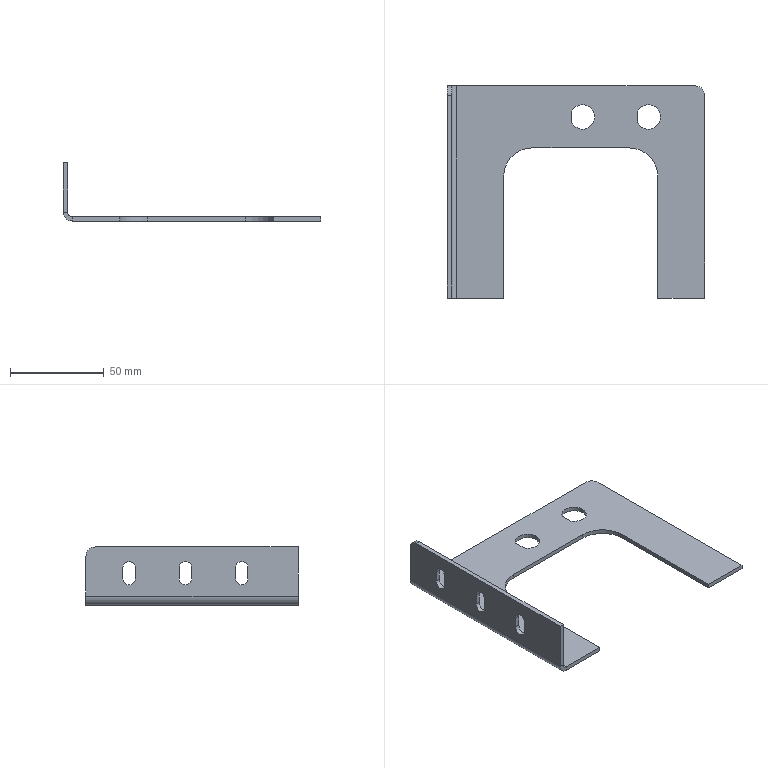Part | SolidWorks | features ICE 2, Fillet 1, FlatPattern 1, SMBaseFlange 1, SheetMetal 1 | 1 solid | 43 faces | box 137 x 113 x 31 mm | volume 26668 mm3 | plane 24 | cylinder 19 | commonest cylinder face diameters 6.6 x9 13 x4 10 x2 30 x2 5 x1 9.6 x1
STEP:
#1=CARTESIAN_POINT('',(2.3,30.,23.25));
#2=VERTEX_POINT('',#1);
#3=CARTESIAN_POINT('',(2.3,33.3,19.95));
#4=VERTEX_POINT('',#3);
#5=CARTESIAN_POINT('',(2.3,30.,19.95));
#6=DIRECTION('',(-1.,0.,0.));
#7=DIRECTION('',(0.,0.,-1.));
#8=AXIS2_PLACEMENT_3D('',#5,#6,#7);
#9=CIRCLE('',#8,3.3);
#10=EDGE_CURVE('',#2,#4,#9,.T.);
#11=ORIENTED_EDGE('',*,*,#10,.F.);
#12=CARTESIAN_POINT('',(0.,30.,23.25));
#13=VERTEX_POINT('',#12);
#14=CARTESIAN_POINT('',(137.001,30.,23.25));
#15=DIRECTION('',(-1.,0.,0.));
#16=VECTOR('',#15,1000.);
#17=LINE('',#14,#16);
#18=EDGE_CURVE('',#2,#13,#17,.T.);
#19=ORIENTED_EDGE('',*,*,#18,.T.);
#20=CARTESIAN_POINT('',(0.,33.3,19.95));
#21=VERTEX_POINT('',#20);
#22=CARTESIAN_POINT('',(0.,30.,19.95));
#23=DIRECTION('',(-1.,0.,0.));
#24=DIRECTION('',(0.,0.,1.));
#25=AXIS2_PLACEMENT_3D('',#22,#23,#24);
#26=CIRCLE('',#25,3.3);
#27=EDGE_CURVE('',#13,#21,#26,.T.);
#28=ORIENTED_EDGE('',*,*,#27,.T.);
#29=CARTESIAN_POINT('',(137.001,33.3,19.95));
#30=DIRECTION('',(-1.,0.,0.));
#31=VECTOR('',#30,1000.);
#32=LINE('',#29,#31);
#33=EDGE_CURVE('',#4,#21,#32,.T.);
#34=ORIENTED_EDGE('',*,*,#33,.F.);
#35=EDGE_LOOP('',(#11,#19,#28,#34));
#36=FACE_OUTER_BOUND('',#35,.T.);
#37=CARTESIAN_POINT('',(137.001,30.,19.95));
#38=DIRECTION('',(-1.,0.,0.));
#39=DIRECTION('',(0.,0.,1.));
#40=AXIS2_PLACEMENT_3D('',#37,#38,#39);
#41=CYLINDRICAL_SURFACE('',#40,3.3);
#42=ADVANCED_FACE('',(#36),#41,.F.);
#43=CARTESIAN_POINT('',(2.3,60.,23.25));
#44=VERTEX_POINT('',#43);
#45=CARTESIAN_POINT('',(2.3,63.3,19.95));
#46=VERTEX_POINT('',#45);
#47=CARTESIAN_POINT('',(2.3,60.,19.95));
#48=DIRECTION('',(-1.,0.,0.));
#49=DIRECTION('',(0.,0.,-1.));
#50=AXIS2_PLACEMENT_3D('',#47,#48,#49);
#51=CIRCLE('',#50,3.3);
#52=EDGE_CURVE('',#44,#46,#51,.T.);
#53=ORIENTED_EDGE('',*,*,#52,.F.);
#54=CARTESIAN_POINT('',(0.,60.,23.25));
#55=VERTEX_POINT('',#54);
#56=CARTESIAN_POINT('',(137.001,60.,23.25));
#57=DIRECTION('',(-1.,0.,0.));
#58=VECTOR('',#57,1000.);
#59=LINE('',#56,#58);
#60=EDGE_CURVE('',#44,#55,#59,.T.);
#61=ORIENTED_EDGE('',*,*,#60,.T.);
#62=CARTESIAN_POINT('',(0.,63.3,19.95));
#63=VERTEX_POINT('',#62);
#64=CARTESIAN_POINT('',(0.,60.,19.95));
#65=DIRECTION('',(-1.,0.,0.));
#66=DIRECTION('',(0.,0.,1.));
#67=AXIS2_PLACEMENT_3D('',#64,#65,#66);
#68=CIRCLE('',#67,3.3);
#69=EDGE_CURVE('',#55,#63,#68,.T.);
#70=ORIENTED_EDGE('',*,*,#69,.T.);
#71=CARTESIAN_POINT('',(137.001,63.3,19.95));
#72=DIRECTION('',(-1.,0.,0.));
#73=VECTOR('',#72,1000.);
#74=LINE('',#71,#73);
#75=EDGE_CURVE('',#46,#63,#74,.T.);
#76=ORIENTED_EDGE('',*,*,#75,.F.);
#77=EDGE_LOOP('',(#53,#61,#70,#76));
#78=FACE_OUTER_BOUND('',#77,.T.);
#79=CARTESIAN_POINT('',(137.001,60.,19.95));
#80=DIRECTION('',(-1.,0.,0.));
#81=DIRECTION('',(0.,0.,1.));
#82=AXIS2_PLACEMENT_3D('',#79,#80,#81);
#83=CYLINDRICAL_SURFACE('',#82,3.3);
#84=ADVANCED_FACE('',(#78),#83,.F.);
#85=CARTESIAN_POINT('',(2.3,90.,23.25));
#86=VERTEX_POINT('',#85);
#87=CARTESIAN_POINT('',(2.3,93.3,19.95));
#88=VERTEX_POINT('',#87);
#89=CARTESIAN_POINT('',(2.3,90.,19.95));
#90=DIRECTION('',(-1.,0.,0.));
#91=DIRECTION('',(0.,0.,-1.));
#92=AXIS2_PLACEMENT_3D('',#89,#90,#91);
#93=CIRCLE('',#92,3.3);
#94=EDGE_CURVE('',#86,#88,#93,.T.);
#95=ORIENTED_EDGE('',*,*,#94,.F.);
#96=CARTESIAN_POINT('',(0.,90.,23.25));
#97=VERTEX_POINT('',#96);
#98=CARTESIAN_POINT('',(137.001,90.,23.25));
#99=DIRECTION('',(-1.,0.,0.));
#100=VECTOR('',#99,1000.);
#101=LINE('',#98,#100);
#102=EDGE_CURVE('',#86,#97,#101,.T.);
#103=ORIENTED_EDGE('',*,*,#102,.T.);
#104=CARTESIAN_POINT('',(0.,93.3,19.95));
#105=VERTEX_POINT('',#104);
#106=CARTESIAN_POINT('',(0.,90.,19.95));
#107=DIRECTION('',(-1.,0.,0.));
#108=DIRECTION('',(0.,0.,1.));
#109=AXIS2_PLACEMENT_3D('',#106,#107,#108);
#110=CIRCLE('',#109,3.3);
#111=EDGE_CURVE('',#97,#105,#110,.T.);
#112=ORIENTED_EDGE('',*,*,#111,.T.);
#113=CARTESIAN_POINT('',(137.001,93.3,19.95));
#114=DIRECTION('',(-1.,0.,0.));
#115=VECTOR('',#114,1000.);
#116=LINE('',#113,#115);
#117=EDGE_CURVE('',#88,#105,#116,.T.);
#118=ORIENTED_EDGE('',*,*,#117,.F.);
#119=EDGE_LOOP('',(#95,#103,#112,#118));
#120=FACE_OUTER_BOUND('',#119,.T.);
#121=CARTESIAN_POINT('',(137.001,90.,19.95));
#122=DIRECTION('',(-1.,0.,0.));
#123=DIRECTION('',(0.,0.,1.));
#124=AXIS2_PLACEMENT_3D('',#121,#122,#123);
#125=CYLINDRICAL_SURFACE('',#124,3.3);
#126=ADVANCED_FACE('',(#120),#125,.F.);
#127=CARTESIAN_POINT('',(101.3,99.624,0.));
#128=VERTEX_POINT('',#127);
#129=CARTESIAN_POINT('',(113.5,96.5,0.));
#130=VERTEX_POINT('',#129);
#131=CARTESIAN_POINT('',(107.,96.5,0.));
#132=DIRECTION('',(0.,0.,-1.));
#133=DIRECTION('',(1.,0.,0.));
#134=AXIS2_PLACEMENT_3D('',#131,#132,#133);
#135=CIRCLE('',#134,6.5);
#136=EDGE_CURVE('',#128,#130,#135,.T.);
#137=ORIENTED_EDGE('',*,*,#136,.T.);
#138=CARTESIAN_POINT('',(113.5,96.5,2.3));
#139=VERTEX_POINT('',#138);
#140=CARTESIAN_POINT('',(113.5,96.5,-0.001));
#141=DIRECTION('',(0.,0.,1.));
#142=VECTOR('',#141,1000.);
#143=LINE('',#140,#142);
#144=EDGE_CURVE('',#130,#139,#143,.T.);
#145=ORIENTED_EDGE('',*,*,#144,.T.);
#146=CARTESIAN_POINT('',(101.3,99.624,2.3));
#147=VERTEX_POINT('',#146);
#148=CARTESIAN_POINT('',(107.,96.5,2.3));
#149=DIRECTION('',(0.,0.,1.));
#150=DIRECTION('',(1.,0.,0.));
#151=AXIS2_PLACEMENT_3D('',#148,#149,#150);
#152=CIRCLE('',#151,6.5);
#153=EDGE_CURVE('',#139,#147,#152,.T.);
#154=ORIENTED_EDGE('',*,*,#153,.T.);
#155=CARTESIAN_POINT('',(101.3,99.624,-0.001));
#156=DIRECTION('',(0.,0.,1.));
#157=VECTOR('',#156,1000.);
#158=LINE('',#155,#157);
#159=EDGE_CURVE('',#128,#147,#158,.T.);
#160=ORIENTED_EDGE('',*,*,#159,.F.);
#161=EDGE_LOOP('',(#137,#145,#154,#160));
#162=FACE_OUTER_BOUND('',#161,.T.);
#163=CARTESIAN_POINT('',(107.,96.5,-0.001));
#164=DIRECTION('',(0.,0.,1.));
#165=DIRECTION('',(1.,0.,0.));
#166=AXIS2_PLACEMENT_3D('',#163,#164,#165);
#167=CYLINDRICAL_SURFACE('',#166,6.5);
#168=ADVANCED_FACE('',(#162),#167,.F.);
#169=CARTESIAN_POINT('',(66.3,99.624,0.));
#170=VERTEX_POINT('',#169);
#171=CARTESIAN_POINT('',(78.5,96.5,0.));
#172=VERTEX_POINT('',#171);
#173=CARTESIAN_POINT('',(72.,96.5,0.));
#174=DIRECTION('',(0.,0.,-1.));
#175=DIRECTION('',(1.,0.,0.));
#176=AXIS2_PLACEMENT_3D('',#173,#174,#175);
#177=CIRCLE('',#176,6.5);
#178=EDGE_CURVE('',#170,#172,#177,.T.);
#179=ORIENTED_EDGE('',*,*,#178,.T.);
#180=CARTESIAN_POINT('',(78.5,96.5,2.3));
#181=VERTEX_POINT('',#180);
#182=CARTESIAN_POINT('',(78.5,96.5,-0.001));
#183=DIRECTION('',(0.,0.,1.));
#184=VECTOR('',#183,1000.);
#185=LINE('',#182,#184);
#186=EDGE_CURVE('',#172,#181,#185,.T.);
#187=ORIENTED_EDGE('',*,*,#186,.T.);
#188=CARTESIAN_POINT('',(66.3,99.624,2.3));
#189=VERTEX_POINT('',#188);
#190=CARTESIAN_POINT('',(72.,96.5,2.3));
#191=DIRECTION('',(0.,0.,1.));
#192=DIRECTION('',(1.,0.,0.));
#193=AXIS2_PLACEMENT_3D('',#190,#191,#192);
#194=CIRCLE('',#193,6.5);
#195=EDGE_CURVE('',#181,#189,#194,.T.);
#196=ORIENTED_EDGE('',*,*,#195,.T.);
#197=CARTESIAN_POINT('',(66.3,99.624,-0.001));
#198=DIRECTION('',(0.,0.,1.));
#199=VECTOR('',#198,1000.);
#200=LINE('',#197,#199);
#201=EDGE_CURVE('',#170,#189,#200,.T.);
#202=ORIENTED_EDGE('',*,*,#201,.F.);
#203=EDGE_LOOP('',(#179,#187,#196,#202));
#204=FACE_OUTER_BOUND('',#203,.T.);
#205=CARTESIAN_POINT('',(72.,96.5,-0.001));
#206=DIRECTION('',(0.,0.,1.));
#207=DIRECTION('',(1.,0.,0.));
#208=AXIS2_PLACEMENT_3D('',#205,#206,#207);
#209=CYLINDRICAL_SURFACE('',#208,6.5);
#210=ADVANCED_FACE('',(#204),#209,.F.);
#211=CARTESIAN_POINT('',(30.,0.,0.));
#212=VERTEX_POINT('',#211);
#213=CARTESIAN_POINT('',(4.8,0.,0.));
#214=VERTEX_POINT('',#213);
#215=CARTESIAN_POINT('',(0.,0.,0.));
#216=DIRECTION('',(-1.,0.,0.));
#217=VECTOR('',#216,1000.);
#218=LINE('',#215,#217);
#219=EDGE_CURVE('',#212,#214,#218,.T.);
#220=ORIENTED_EDGE('',*,*,#219,.F.);
#221=CARTESIAN_POINT('',(30.,0.,2.3));
#222=VERTEX_POINT('',#221);
#223=CARTESIAN_POINT('',(30.,0.,-0.001));
#224=DIRECTION('',(0.,0.,1.));
#225=VECTOR('',#224,1000.);
#226=LINE('',#223,#225);
#227=EDGE_CURVE('',#212,#222,#226,.T.);
#228=ORIENTED_EDGE('',*,*,#227,.T.);
#229=CARTESIAN_POINT('',(4.8,0.,2.3));
#230=VERTEX_POINT('',#229);
#231=CARTESIAN_POINT('',(0.,0.,2.3));
#232=DIRECTION('',(-1.,0.,0.));
#233=VECTOR('',#232,1000.);
#234=LINE('',#231,#233);
#235=EDGE_CURVE('',#222,#230,#234,.T.);
#236=ORIENTED_EDGE('',*,*,#235,.T.);
#237=CARTESIAN_POINT('',(4.8,0.,2.3));
#238=DIRECTION('',(0.,0.,-1.));
#239=VECTOR('',#238,1000.);
#240=LINE('',#237,#239);
#241=EDGE_CURVE('',#230,#214,#240,.T.);
#242=ORIENTED_EDGE('',*,*,#241,.T.);
#243=EDGE_LOOP('',(#220,#228,#236,#242));
#244=FACE_OUTER_BOUND('',#243,.T.);
#245=CARTESIAN_POINT('',(4.8,0.,4.8));
#246=DIRECTION('',(0.,1.,0.));
#247=DIRECTION('',(1.,0.,0.));
#248=AXIS2_PLACEMENT_3D('',#245,#246,#247);
#249=PLANE('',#248);
#250=ADVANCED_FACE('',(#244),#249,.F.);
#251=CARTESIAN_POINT('',(4.8,113.,0.));
#252=VERTEX_POINT('',#251);
#253=CARTESIAN_POINT('',(4.8,113.,2.3));
#254=VERTEX_POINT('',#253);
#255=CARTESIAN_POINT('',(4.8,113.,0.));
#256=DIRECTION('',(0.,0.,1.));
#257=VECTOR('',#256,1000.);
#258=LINE('',#255,#257);
#259=EDGE_CURVE('',#252,#254,#258,.T.);
#260=ORIENTED_EDGE('',*,*,#259,.F.);
#261=CARTESIAN_POINT('',(0.,113.,4.8));
#262=VERTEX_POINT('',#261);
#263=CARTESIAN_POINT('',(4.8,113.,4.8));
#264=DIRECTION('',(0.,1.,0.));
#265=DIRECTION('',(0.,0.,-1.));
#266=AXIS2_PLACEMENT_3D('',#263,#264,#265);
#267=CIRCLE('',#266,4.8);
#268=EDGE_CURVE('',#252,#262,#267,.T.);
#269=ORIENTED_EDGE('',*,*,#268,.T.);
#270=CARTESIAN_POINT('',(2.3,113.,4.8));
#271=VERTEX_POINT('',#270);
#272=CARTESIAN_POINT('',(2.3,113.,4.8));
#273=DIRECTION('',(-1.,0.,0.));
#274=VECTOR('',#273,1000.);
#275=LINE('',#272,#274);
#276=EDGE_CURVE('',#271,#262,#275,.T.);
#277=ORIENTED_EDGE('',*,*,#276,.F.);
#278=CARTESIAN_POINT('',(4.8,113.,4.8));
#279=DIRECTION('',(0.,1.,0.));
#280=DIRECTION('',(1.,0.,0.));
#281=AXIS2_PLACEMENT_3D('',#278,#279,#280);
#282=CIRCLE('',#281,2.5);
#283=EDGE_CURVE('',#254,#271,#282,.T.);
#284=ORIENTED_EDGE('',*,*,#283,.F.);
#285=EDGE_LOOP('',(#260,#269,#277,#284));
#286=FACE_OUTER_BOUND('',#285,.T.);
#287=CARTESIAN_POINT('',(4.8,113.,0.));
#288=DIRECTION('',(0.,1.,0.));
#289=DIRECTION('',(0.,0.,1.));
#290=AXIS2_PLACEMENT_3D('',#287,#288,#289);
#291=PLANE('',#290);
#292=ADVANCED_FACE('',(#286),#291,.T.);
#293=CARTESIAN_POINT('',(132.,113.,2.3));
#294=VERTEX_POINT('',#293);
#295=CARTESIAN_POINT('',(0.,113.,2.3));
#296=DIRECTION('',(-1.,0.,0.));
#297=VECTOR('',#296,1000.);
#298=LINE('',#295,#297);
#299=EDGE_CURVE('',#294,#254,#298,.T.);
#300=ORIENTED_EDGE('',*,*,#299,.F.);
#301=CARTESIAN_POINT('',(132.,113.,0.));
#302=VERTEX_POINT('',#301);
#303=CARTESIAN_POINT('',(132.,113.,4.8));
#304=DIRECTION('',(0.,0.,-1.));
#305=VECTOR('',#304,1000.);
#306=LINE('',#303,#305);
#307=EDGE_CURVE('',#294,#302,#306,.T.);
#308=ORIENTED_EDGE('',*,*,#307,.T.);
#309=CARTESIAN_POINT('',(0.,113.,0.));
#310=DIRECTION('',(-1.,0.,0.));
#311=VECTOR('',#310,1000.);
#312=LINE('',#309,#311);
#313=EDGE_CURVE('',#302,#252,#312,.T.);
#314=ORIENTED_EDGE('',*,*,#313,.T.);
#315=ORIENTED_EDGE('',*,*,#259,.T.);
#316=EDGE_LOOP('',(#300,#308,#314,#315));
#317=FACE_OUTER_BOUND('',#316,.T.);
#318=CARTESIAN_POINT('',(2.3,113.,4.8));
#319=DIRECTION('',(0.,1.,0.));
#320=DIRECTION('',(0.,0.,1.));
#321=AXIS2_PLACEMENT_3D('',#318,#319,#320);
#322=PLANE('',#321);
#323=ADVANCED_FACE('',(#317),#322,.T.);
#324=CARTESIAN_POINT('',(0.,0.,4.8));
#325=VERTEX_POINT('',#324);
#326=CARTESIAN_POINT('',(2.3,0.,4.8));
#327=VERTEX_POINT('',#326);
#328=CARTESIAN_POINT('',(0.,0.,4.8));
#329=DIRECTION('',(1.,0.,0.));
#330=VECTOR('',#329,1000.);
#331=LINE('',#328,#330);
#332=EDGE_CURVE('',#325,#327,#331,.T.);
#333=ORIENTED_EDGE('',*,*,#332,.F.);
#334=CARTESIAN_POINT('',(4.8,0.,4.8));
#335=DIRECTION('',(0.,1.,0.));
#336=DIRECTION('',(0.,0.,-1.));
#337=AXIS2_PLACEMENT_3D('',#334,#335,#336);
#338=CIRCLE('',#337,4.8);
#339=EDGE_CURVE('',#214,#325,#338,.T.);
#340=ORIENTED_EDGE('',*,*,#339,.F.);
#341=ORIENTED_EDGE('',*,*,#241,.F.);
#342=CARTESIAN_POINT('',(4.8,0.,4.8));
#343=DIRECTION('',(0.,1.,0.));
#344=DIRECTION('',(1.,0.,0.));
#345=AXIS2_PLACEMENT_3D('',#342,#343,#344);
#346=CIRCLE('',#345,2.5);
#347=EDGE_CURVE('',#230,#327,#346,.T.);
#348=ORIENTED_EDGE('',*,*,#347,.T.);
#349=EDGE_LOOP('',(#333,#340,#341,#348));
#350=FACE_OUTER_BOUND('',#349,.T.);
#351=CARTESIAN_POINT('',(0.,0.,4.8));
#352=DIRECTION('',(0.,-1.,0.));
#353=DIRECTION('',(0.,0.,-1.));
#354=AXIS2_PLACEMENT_3D('',#351,#352,#353);
#355=PLANE('',#354);
#356=ADVANCED_FACE('',(#350),#355,.T.);
#357=CARTESIAN_POINT('',(0.,0.,31.));
#358=VERTEX_POINT('',#357);
#359=CARTESIAN_POINT('',(0.,0.,0.));
#360=DIRECTION('',(0.,0.,1.));
#361=VECTOR('',#360,1000.);
#362=LINE('',#359,#361);
#363=EDGE_CURVE('',#325,#358,#362,.T.);
#364=ORIENTED_EDGE('',*,*,#363,.F.);
#365=ORIENTED_EDGE('',*,*,#332,.T.);
#366=CARTESIAN_POINT('',(2.3,0.,31.));
#367=VERTEX_POINT('',#366);
#368=CARTESIAN_POINT('',(2.3,0.,0.));
#369=DIRECTION('',(0.,0.,1.));
#370=VECTOR('',#369,1000.);
#371=LINE('',#368,#370);
#372=EDGE_CURVE('',#327,#367,#371,.T.);
#373=ORIENTED_EDGE('',*,*,#372,.T.);
#374=CARTESIAN_POINT('',(2.3,0.,31.));
#375=DIRECTION('',(-1.,0.,0.));
#376=VECTOR('',#375,1000.);
#377=LINE('',#374,#376);
#378=EDGE_CURVE('',#367,#358,#377,.T.);
#379=ORIENTED_EDGE('',*,*,#378,.T.);
#380=EDGE_LOOP('',(#364,#365,#373,#379));
#381=FACE_OUTER_BOUND('',#380,.T.);
#382=CARTESIAN_POINT('',(4.8,0.,2.3));
#383=DIRECTION('',(0.,-1.,0.));
#384=DIRECTION('',(0.,0.,-1.));
#385=AXIS2_PLACEMENT_3D('',#382,#383,#384);
#386=PLANE('',#385);
#387=ADVANCED_FACE('',(#381),#386,.T.);
#388=CARTESIAN_POINT('',(0.,26.7,14.05));
#389=VERTEX_POINT('',#388);
#390=CARTESIAN_POINT('',(0.,26.7,19.95));
#391=VERTEX_POINT('',#390);
#392=CARTESIAN_POINT('',(0.,26.7,14.05));
#393=DIRECTION('',(0.,0.,1.));
#394=VECTOR('',#393,1000.);
#395=LINE('',#392,#394);
#396=EDGE_CURVE('',#389,#391,#395,.T.);
#397=ORIENTED_EDGE('',*,*,#396,.F.);
#398=CARTESIAN_POINT('',(0.,33.3,14.05));
#399=VERTEX_POINT('',#398);
#400=CARTESIAN_POINT('',(0.,30.,14.05));
#401=DIRECTION('',(-1.,0.,0.));
#402=DIRECTION('',(0.,0.,1.));
#403=AXIS2_PLACEMENT_3D('',#400,#401,#402);
#404=CIRCLE('',#403,3.3);
#405=EDGE_CURVE('',#399,#389,#404,.T.);
#406=ORIENTED_EDGE('',*,*,#405,.F.);
#407=CARTESIAN_POINT('',(0.,33.3,14.05));
#408=DIRECTION('',(0.,0.,-1.));
#409=VECTOR('',#408,1000.);
#410=LINE('',#407,#409);
#411=EDGE_CURVE('',#21,#399,#410,.T.);
#412=ORIENTED_EDGE('',*,*,#411,.F.);
#413=ORIENTED_EDGE('',*,*,#27,.F.);
#414=CARTESIAN_POINT('',(0.,30.,19.95));
#415=DIRECTION('',(-1.,0.,0.));
#416=DIRECTION('',(0.,0.,1.));
#417=AXIS2_PLACEMENT_3D('',#414,#415,#416);
#418=CIRCLE('',#417,3.3);
#419=EDGE_CURVE('',#391,#13,#418,.T.);
#420=ORIENTED_EDGE('',*,*,#419,.F.);
#421=EDGE_LOOP('',(#397,#406,#412,#413,#420));
#422=FACE_BOUND('',#421,.T.);
#423=CARTESIAN_POINT('',(0.,56.7,14.05));
#424=VERTEX_POINT('',#423);
#425=CARTESIAN_POINT('',(0.,56.7,19.95));
#426=VERTEX_POINT('',#425);
#427=CARTESIAN_POINT('',(0.,56.7,14.05));
#428=DIRECTION('',(0.,0.,1.));
#429=VECTOR('',#428,1000.);
#430=LINE('',#427,#429);
#431=EDGE_CURVE('',#424,#426,#430,.T.);
#432=ORIENTED_EDGE('',*,*,#431,.F.);
#433=CARTESIAN_POINT('',(0.,63.3,14.05));
#434=VERTEX_POINT('',#433);
#435=CARTESIAN_POINT('',(0.,60.,14.05));
#436=DIRECTION('',(-1.,0.,0.));
#437=DIRECTION('',(0.,0.,1.));
#438=AXIS2_PLACEMENT_3D('',#435,#436,#437);
#439=CIRCLE('',#438,3.3);
#440=EDGE_CURVE('',#434,#424,#439,.T.);
#441=ORIENTED_EDGE('',*,*,#440,.F.);
#442=CARTESIAN_POINT('',(0.,63.3,14.05));
#443=DIRECTION('',(0.,0.,-1.));
#444=VECTOR('',#443,1000.);
#445=LINE('',#442,#444);
#446=EDGE_CURVE('',#63,#434,#445,.T.);
#447=ORIENTED_EDGE('',*,*,#446,.F.);
#448=ORIENTED_EDGE('',*,*,#69,.F.);
#449=CARTESIAN_POINT('',(0.,60.,19.95));
#450=DIRECTION('',(-1.,0.,0.));
#451=DIRECTION('',(0.,0.,1.));
#452=AXIS2_PLACEMENT_3D('',#449,#450,#451);
#453=CIRCLE('',#452,3.3);
#454=EDGE_CURVE('',#426,#55,#453,.T.);
#455=ORIENTED_EDGE('',*,*,#454,.F.);
#456=EDGE_LOOP('',(#432,#441,#447,#448,#455));
#457=FACE_BOUND('',#456,.T.);
#458=CARTESIAN_POINT('',(0.,86.7,14.05));
#459=VERTEX_POINT('',#458);
#460=CARTESIAN_POINT('',(0.,86.7,19.95));
#461=VERTEX_POINT('',#460);
#462=CARTESIAN_POINT('',(0.,86.7,14.05));
#463=DIRECTION('',(0.,0.,1.));
#464=VECTOR('',#463,1000.);
#465=LINE('',#462,#464);
#466=EDGE_CURVE('',#459,#461,#465,.T.);
#467=ORIENTED_EDGE('',*,*,#466,.F.);
#468=CARTESIAN_POINT('',(0.,93.3,14.05));
#469=VERTEX_POINT('',#468);
#470=CARTESIAN_POINT('',(0.,90.,14.05));
#471=DIRECTION('',(-1.,0.,0.));
#472=DIRECTION('',(0.,0.,1.));
#473=AXIS2_PLACEMENT_3D('',#470,#471,#472);
#474=CIRCLE('',#473,3.3);
#475=EDGE_CURVE('',#469,#459,#474,.T.);
#476=ORIENTED_EDGE('',*,*,#475,.F.);
#477=CARTESIAN_POINT('',(0.,93.3,14.05));
#478=DIRECTION('',(0.,0.,-1.));
#479=VECTOR('',#478,1000.);
#480=LINE('',#477,#479);
#481=EDGE_CURVE('',#105,#469,#480,.T.);
#482=ORIENTED_EDGE('',*,*,#481,.F.);
#483=ORIENTED_EDGE('',*,*,#111,.F.);
#484=CARTESIAN_POINT('',(0.,90.,19.95));
#485=DIRECTION('',(-1.,0.,0.));
#486=DIRECTION('',(0.,0.,1.));
#487=AXIS2_PLACEMENT_3D('',#484,#485,#486);
#488=CIRCLE('',#487,3.3);
#489=EDGE_CURVE('',#461,#97,#488,.T.);
#490=ORIENTED_EDGE('',*,*,#489,.F.);
#491=EDGE_LOOP('',(#467,#476,#482,#483,#490));
#492=FACE_BOUND('',#491,.T.);
#493=CARTESIAN_POINT('',(0.,108.,31.));
#494=VERTEX_POINT('',#493);
#495=CARTESIAN_POINT('',(0.,113.,31.));
#496=DIRECTION('',(0.,-1.,0.));
#497=VECTOR('',#496,1000.);
#498=LINE('',#495,#497);
#499=EDGE_CURVE('',#494,#358,#498,.T.);
#500=ORIENTED_EDGE('',*,*,#499,.F.);
#501=CARTESIAN_POINT('',(0.,113.,26.));
#502=VERTEX_POINT('',#501);
#503=CARTESIAN_POINT('',(0.,108.,26.));
#504=DIRECTION('',(-1.,0.,0.));
#505=DIRECTION('',(0.,0.,-1.));
#506=AXIS2_PLACEMENT_3D('',#503,#504,#505);
#507=CIRCLE('',#506,5.);
#508=EDGE_CURVE('',#494,#502,#507,.T.);
#509=ORIENTED_EDGE('',*,*,#508,.T.);
#510=CARTESIAN_POINT('',(0.,113.,0.));
#511=DIRECTION('',(0.,0.,1.));
#512=VECTOR('',#511,1000.);
#513=LINE('',#510,#512);
#514=EDGE_CURVE('',#262,#502,#513,.T.);
#515=ORIENTED_EDGE('',*,*,#514,.F.);
#516=CARTESIAN_POINT('',(0.,113.,4.8));
#517=DIRECTION('',(0.,-1.,0.));
#518=VECTOR('',#517,1000.);
#519=LINE('',#516,#518);
#520=EDGE_CURVE('',#262,#325,#519,.T.);
#521=ORIENTED_EDGE('',*,*,#520,.T.);
#522=ORIENTED_EDGE('',*,*,#363,.T.);
#523=EDGE_LOOP('',(#500,#509,#515,#521,#522));
#524=FACE_OUTER_BOUND('',#523,.T.);
#525=CARTESIAN_POINT('',(0.,113.,0.));
#526=DIRECTION('',(1.,0.,0.));
#527=DIRECTION('',(0.,0.,-1.));
#528=AXIS2_PLACEMENT_3D('',#525,#526,#527);
#529=PLANE('',#528);
#530=ADVANCED_FACE('',(#422,#457,#492,#524),#529,.F.);
#531=CARTESIAN_POINT('',(2.3,108.,31.));
#532=VERTEX_POINT('',#531);
#533=CARTESIAN_POINT('',(2.3,113.,31.));
#534=DIRECTION('',(0.,-1.,0.));
#535=VECTOR('',#534,1000.);
#536=LINE('',#533,#535);
#537=EDGE_CURVE('',#532,#367,#536,.T.);
#538=ORIENTED_EDGE('',*,*,#537,.F.);
#539=CARTESIAN_POINT('',(2.3,108.,31.));
#540=DIRECTION('',(-1.,0.,0.));
#541=VECTOR('',#540,1000.);
#542=LINE('',#539,#541);
#543=EDGE_CURVE('',#532,#494,#542,.T.);
#544=ORIENTED_EDGE('',*,*,#543,.T.);
#545=ORIENTED_EDGE('',*,*,#499,.T.);
#546=ORIENTED_EDGE('',*,*,#378,.F.);
#547=EDGE_LOOP('',(#538,#544,#545,#546));
#548=FACE_OUTER_BOUND('',#547,.T.);
#549=CARTESIAN_POINT('',(2.3,113.,31.));
#550=DIRECTION('',(0.,0.,1.));
#551=DIRECTION('',(1.,0.,0.));
#552=AXIS2_PLACEMENT_3D('',#549,#550,#551);
#553=PLANE('',#552);
#554=ADVANCED_FACE('',(#548),#553,.T.);
#555=CARTESIAN_POINT('',(2.3,33.3,14.05));
#556=VERTEX_POINT('',#555);
#557=CARTESIAN_POINT('',(2.3,26.7,14.05));
#558=VERTEX_POINT('',#557);
#559=CARTESIAN_POINT('',(2.3,30.,14.05));
#560=DIRECTION('',(-1.,0.,0.));
#561=DIRECTION('',(0.,0.,-1.));
#562=AXIS2_PLACEMENT_3D('',#559,#560,#561);
#563=CIRCLE('',#562,3.3);
#564=EDGE_CURVE('',#556,#558,#563,.T.);
#565=ORIENTED_EDGE('',*,*,#564,.T.);
#566=CARTESIAN_POINT('',(2.3,26.7,19.95));
#567=VERTEX_POINT('',#566);
#568=CARTESIAN_POINT('',(2.3,26.7,14.05));
#569=DIRECTION('',(0.,0.,1.));
#570=VECTOR('',#569,1000.);
#571=LINE('',#568,#570);
#572=EDGE_CURVE('',#558,#567,#571,.T.);
#573=ORIENTED_EDGE('',*,*,#572,.T.);
#574=CARTESIAN_POINT('',(2.3,30.,19.95));
#575=DIRECTION('',(-1.,0.,0.));
#576=DIRECTION('',(0.,0.,-1.));
#577=AXIS2_PLACEMENT_3D('',#574,#575,#576);
#578=CIRCLE('',#577,3.3);
#579=EDGE_CURVE('',#567,#2,#578,.T.);
#580=ORIENTED_EDGE('',*,*,#579,.T.);
#581=ORIENTED_EDGE('',*,*,#10,.T.);
#582=CARTESIAN_POINT('',(2.3,33.3,14.05));
#583=DIRECTION('',(0.,0.,-1.));
#584=VECTOR('',#583,1000.);
#585=LINE('',#582,#584);
#586=EDGE_CURVE('',#4,#556,#585,.T.);
#587=ORIENTED_EDGE('',*,*,#586,.T.);
#588=EDGE_LOOP('',(#565,#573,#580,#581,#587));
#589=FACE_BOUND('',#588,.T.);
#590=CARTESIAN_POINT('',(2.3,63.3,14.05));
#591=VERTEX_POINT('',#590);
#592=CARTESIAN_POINT('',(2.3,56.7,14.05));
#593=VERTEX_POINT('',#592);
#594=CARTESIAN_POINT('',(2.3,60.,14.05));
#595=DIRECTION('',(-1.,0.,0.));
#596=DIRECTION('',(0.,0.,-1.));
#597=AXIS2_PLACEMENT_3D('',#594,#595,#596);
#598=CIRCLE('',#597,3.3);
#599=EDGE_CURVE('',#591,#593,#598,.T.);
#600=ORIENTED_EDGE('',*,*,#599,.T.);
#601=CARTESIAN_POINT('',(2.3,56.7,19.95));
#602=VERTEX_POINT('',#601);
#603=CARTESIAN_POINT('',(2.3,56.7,14.05));
#604=DIRECTION('',(0.,0.,1.));
#605=VECTOR('',#604,1000.);
#606=LINE('',#603,#605);
#607=EDGE_CURVE('',#593,#602,#606,.T.);
#608=ORIENTED_EDGE('',*,*,#607,.T.);
#609=CARTESIAN_POINT('',(2.3,60.,19.95));
#610=DIRECTION('',(-1.,0.,0.));
#611=DIRECTION('',(0.,0.,-1.));
#612=AXIS2_PLACEMENT_3D('',#609,#610,#611);
#613=CIRCLE('',#612,3.3);
#614=EDGE_CURVE('',#602,#44,#613,.T.);
#615=ORIENTED_EDGE('',*,*,#614,.T.);
#616=ORIENTED_EDGE('',*,*,#52,.T.);
#617=CARTESIAN_POINT('',(2.3,63.3,14.05));
#618=DIRECTION('',(0.,0.,-1.));
#619=VECTOR('',#618,1000.);
#620=LINE('',#617,#619);
#621=EDGE_CURVE('',#46,#591,#620,.T.);
#622=ORIENTED_EDGE('',*,*,#621,.T.);
#623=EDGE_LOOP('',(#600,#608,#615,#616,#622));
#624=FACE_BOUND('',#623,.T.);
#625=CARTESIAN_POINT('',(2.3,93.3,14.05));
#626=VERTEX_POINT('',#625);
#627=CARTESIAN_POINT('',(2.3,86.7,14.05));
#628=VERTEX_POINT('',#627);
#629=CARTESIAN_POINT('',(2.3,90.,14.05));
#630=DIRECTION('',(-1.,0.,0.));
#631=DIRECTION('',(0.,0.,-1.));
#632=AXIS2_PLACEMENT_3D('',#629,#630,#631);
#633=CIRCLE('',#632,3.3);
#634=EDGE_CURVE('',#626,#628,#633,.T.);
#635=ORIENTED_EDGE('',*,*,#634,.T.);
#636=CARTESIAN_POINT('',(2.3,86.7,19.95));
#637=VERTEX_POINT('',#636);
#638=CARTESIAN_POINT('',(2.3,86.7,14.05));
#639=DIRECTION('',(0.,0.,1.));
#640=VECTOR('',#639,1000.);
#641=LINE('',#638,#640);
#642=EDGE_CURVE('',#628,#637,#641,.T.);
#643=ORIENTED_EDGE('',*,*,#642,.T.);
#644=CARTESIAN_POINT('',(2.3,90.,19.95));
#645=DIRECTION('',(-1.,0.,0.));
#646=DIRECTION('',(0.,0.,-1.));
#647=AXIS2_PLACEMENT_3D('',#644,#645,#646);
#648=CIRCLE('',#647,3.3);
#649=EDGE_CURVE('',#637,#86,#648,.T.);
#650=ORIENTED_EDGE('',*,*,#649,.T.);
#651=ORIENTED_EDGE('',*,*,#94,.T.);
#652=CARTESIAN_POINT('',(2.3,93.3,14.05));
#653=DIRECTION('',(0.,0.,-1.));
#654=VECTOR('',#653,1000.);
#655=LINE('',#652,#654);
#656=EDGE_CURVE('',#88,#626,#655,.T.);
#657=ORIENTED_EDGE('',*,*,#656,.T.);
#658=EDGE_LOOP('',(#635,#643,#650,#651,#657));
#659=FACE_BOUND('',#658,.T.);
#660=CARTESIAN_POINT('',(2.3,113.,26.));
#661=VERTEX_POINT('',#660);
#662=CARTESIAN_POINT('',(2.3,113.,0.));
#663=DIRECTION('',(0.,0.,1.));
#664=VECTOR('',#663,1000.);
#665=LINE('',#662,#664);
#666=EDGE_CURVE('',#271,#661,#665,.T.);
#667=ORIENTED_EDGE('',*,*,#666,.T.);
#668=CARTESIAN_POINT('',(2.3,108.,26.));
#669=DIRECTION('',(1.,0.,0.));
#670=DIRECTION('',(0.,0.,-1.));
#671=AXIS2_PLACEMENT_3D('',#668,#669,#670);
#672=CIRCLE('',#671,5.);
#673=EDGE_CURVE('',#661,#532,#672,.T.);
#674=ORIENTED_EDGE('',*,*,#673,.T.);
#675=ORIENTED_EDGE('',*,*,#537,.T.);
#676=ORIENTED_EDGE('',*,*,#372,.F.);
#677=CARTESIAN_POINT('',(2.3,113.,4.8));
#678=DIRECTION('',(0.,-1.,0.));
#679=VECTOR('',#678,1000.);
#680=LINE('',#677,#679);
#681=EDGE_CURVE('',#271,#327,#680,.T.);
#682=ORIENTED_EDGE('',*,*,#681,.F.);
#683=EDGE_LOOP('',(#667,#674,#675,#676,#682));
#684=FACE_OUTER_BOUND('',#683,.T.);
#685=CARTESIAN_POINT('',(2.3,113.,0.));
#686=DIRECTION('',(1.,0.,0.));
#687=DIRECTION('',(0.,0.,-1.));
#688=AXIS2_PLACEMENT_3D('',#685,#686,#687);
#689=PLANE('',#688);
#690=ADVANCED_FACE('',(#589,#624,#659,#684),#689,.T.);
#691=ORIENTED_EDGE('',*,*,#347,.F.);
#692=CARTESIAN_POINT('',(4.8,113.,2.3));
#693=DIRECTION('',(0.,-1.,0.));
#694=VECTOR('',#693,1000.);
#695=LINE('',#692,#694);
#696=EDGE_CURVE('',#254,#230,#695,.T.);
#697=ORIENTED_EDGE('',*,*,#696,.F.);
#698=ORIENTED_EDGE('',*,*,#283,.T.);
#699=ORIENTED_EDGE('',*,*,#681,.T.);
#700=EDGE_LOOP('',(#691,#697,#698,#699));
#701=FACE_OUTER_BOUND('',#700,.T.);
#702=CARTESIAN_POINT('',(4.8,113.,4.8));
#703=DIRECTION('',(0.,-1.,0.));
#704=DIRECTION('',(0.,0.,-1.));
#705=AXIS2_PLACEMENT_3D('',#702,#703,#704);
#706=CYLINDRICAL_SURFACE('',#705,2.5);
#707=ADVANCED_FACE('',(#701),#706,.F.);
#708=CARTESIAN_POINT('',(137.,108.,2.3));
#709=VERTEX_POINT('',#708);
#710=CARTESIAN_POINT('',(137.,0.,2.3));
#711=VERTEX_POINT('',#710);
#712=CARTESIAN_POINT('',(137.,113.,2.3));
#713=DIRECTION('',(0.,-1.,0.));
#714=VECTOR('',#713,1000.);
#715=LINE('',#712,#714);
#716=EDGE_CURVE('',#709,#711,#715,.T.);
#717=ORIENTED_EDGE('',*,*,#716,.F.);
#718=CARTESIAN_POINT('',(132.,108.,2.3));
#719=DIRECTION('',(0.,0.,1.));
#720=DIRECTION('',(1.,0.,0.));
#721=AXIS2_PLACEMENT_3D('',#718,#719,#720);
#722=CIRCLE('',#721,5.);
#723=EDGE_CURVE('',#709,#294,#722,.T.);
#724=ORIENTED_EDGE('',*,*,#723,.T.);
#725=ORIENTED_EDGE('',*,*,#299,.T.);
#726=ORIENTED_EDGE('',*,*,#696,.T.);
#727=ORIENTED_EDGE('',*,*,#235,.F.);
#728=CARTESIAN_POINT('',(30.,65.,2.3));
#729=VERTEX_POINT('',#728);
#730=CARTESIAN_POINT('',(30.,0.,2.3));
#731=DIRECTION('',(0.,-1.,0.));
#732=VECTOR('',#731,1000.);
#733=LINE('',#730,#732);
#734=EDGE_CURVE('',#729,#222,#733,.T.);
#735=ORIENTED_EDGE('',*,*,#734,.F.);
#736=CARTESIAN_POINT('',(45.,80.,2.3));
#737=VERTEX_POINT('',#736);
#738=CARTESIAN_POINT('',(45.,65.,2.3));
#739=DIRECTION('',(0.,0.,1.));
#740=DIRECTION('',(-1.,0.,0.));
#741=AXIS2_PLACEMENT_3D('',#738,#739,#740);
#742=CIRCLE('',#741,15.);
#743=EDGE_CURVE('',#737,#729,#742,.T.);
#744=ORIENTED_EDGE('',*,*,#743,.F.);
#745=CARTESIAN_POINT('',(97.,80.,2.3));
#746=VERTEX_POINT('',#745);
#747=CARTESIAN_POINT('',(45.,80.,2.3));
#748=DIRECTION('',(-1.,0.,0.));
#749=VECTOR('',#748,1000.);
#750=LINE('',#747,#749);
#751=EDGE_CURVE('',#746,#737,#750,.T.);
#752=ORIENTED_EDGE('',*,*,#751,.F.);
#753=CARTESIAN_POINT('',(112.,65.,2.3));
#754=VERTEX_POINT('',#753);
#755=CARTESIAN_POINT('',(97.,65.,2.3));
#756=DIRECTION('',(0.,0.,1.));
#757=DIRECTION('',(-1.,0.,0.));
#758=AXIS2_PLACEMENT_3D('',#755,#756,#757);
#759=CIRCLE('',#758,15.);
#760=EDGE_CURVE('',#754,#746,#759,.T.);
#761=ORIENTED_EDGE('',*,*,#760,.F.);
#762=CARTESIAN_POINT('',(112.,0.,2.3));
#763=VERTEX_POINT('',#762);
#764=CARTESIAN_POINT('',(112.,65.,2.3));
#765=DIRECTION('',(0.,1.,0.));
#766=VECTOR('',#765,1000.);
#767=LINE('',#764,#766);
#768=EDGE_CURVE('',#763,#754,#767,.T.);
#769=ORIENTED_EDGE('',*,*,#768,.F.);
#770=CARTESIAN_POINT('',(0.,0.,2.3));
#771=DIRECTION('',(-1.,0.,0.));
#772=VECTOR('',#771,1000.);
#773=LINE('',#770,#772);
#774=EDGE_CURVE('',#711,#763,#773,.T.);
#775=ORIENTED_EDGE('',*,*,#774,.F.);
#776=EDGE_LOOP('',(#717,#724,#725,#726,#727,#735,#744,#752,#761,#769,#775));
#777=FACE_OUTER_BOUND('',#776,.T.);
#778=CARTESIAN_POINT('',(101.3,93.376,2.3));
#779=VERTEX_POINT('',#778);
#780=CARTESIAN_POINT('',(107.,96.5,2.3));
#781=DIRECTION('',(0.,0.,1.));
#782=DIRECTION('',(1.,0.,0.));
#783=AXIS2_PLACEMENT_3D('',#780,#781,#782);
#784=CIRCLE('',#783,6.5);
#785=EDGE_CURVE('',#779,#139,#784,.T.);
#786=ORIENTED_EDGE('',*,*,#785,.F.);
#787=CARTESIAN_POINT('',(101.3,93.376,2.3));
#788=DIRECTION('',(0.,-1.,0.));
#789=VECTOR('',#788,1000.);
#790=LINE('',#787,#789);
#791=EDGE_CURVE('',#147,#779,#790,.T.);
#792=ORIENTED_EDGE('',*,*,#791,.F.);
#793=ORIENTED_EDGE('',*,*,#153,.F.);
#794=EDGE_LOOP('',(#786,#792,#793));
#795=FACE_BOUND('',#794,.T.);
#796=CARTESIAN_POINT('',(66.3,93.376,2.3));
#797=VERTEX_POINT('',#796);
#798=CARTESIAN_POINT('',(72.,96.5,2.3));
#799=DIRECTION('',(0.,0.,1.));
#800=DIRECTION('',(1.,0.,0.));
#801=AXIS2_PLACEMENT_3D('',#798,#799,#800);
#802=CIRCLE('',#801,6.5);
#803=EDGE_CURVE('',#797,#181,#802,.T.);
#804=ORIENTED_EDGE('',*,*,#803,.F.);
#805=CARTESIAN_POINT('',(66.3,99.624,2.3));
#806=DIRECTION('',(0.,-1.,0.));
#807=VECTOR('',#806,1000.);
#808=LINE('',#805,#807);
#809=EDGE_CURVE('',#189,#797,#808,.T.);
#810=ORIENTED_EDGE('',*,*,#809,.F.);
#811=ORIENTED_EDGE('',*,*,#195,.F.);
#812=EDGE_LOOP('',(#804,#810,#811));
#813=FACE_BOUND('',#812,.T.);
#814=CARTESIAN_POINT('',(0.,113.,2.3));
#815=DIRECTION('',(0.,0.,1.));
#816=DIRECTION('',(1.,0.,0.));
#817=AXIS2_PLACEMENT_3D('',#814,#815,#816);
#818=PLANE('',#817);
#819=ADVANCED_FACE('',(#777,#795,#813),#818,.T.);
#820=CARTESIAN_POINT('',(137.,108.,0.));
#821=VERTEX_POINT('',#820);
#822=CARTESIAN_POINT('',(137.,0.,0.));
#823=VERTEX_POINT('',#822);
#824=CARTESIAN_POINT('',(137.,113.,0.));
#825=DIRECTION('',(0.,-1.,0.));
#826=VECTOR('',#825,1000.);
#827=LINE('',#824,#826);
#828=EDGE_CURVE('',#821,#823,#827,.T.);
#829=ORIENTED_EDGE('',*,*,#828,.F.);
#830=CARTESIAN_POINT('',(137.,108.,0.));
#831=DIRECTION('',(0.,0.,1.));
#832=VECTOR('',#831,1000.);
#833=LINE('',#830,#832);
#834=EDGE_CURVE('',#821,#709,#833,.T.);
#835=ORIENTED_EDGE('',*,*,#834,.T.);
#836=ORIENTED_EDGE('',*,*,#716,.T.);
#837=CARTESIAN_POINT('',(137.,0.,0.));
#838=DIRECTION('',(0.,0.,1.));
#839=VECTOR('',#838,1000.);
#840=LINE('',#837,#839);
#841=EDGE_CURVE('',#823,#711,#840,.T.);
#842=ORIENTED_EDGE('',*,*,#841,.F.);
#843=EDGE_LOOP('',(#829,#835,#836,#842));
#844=FACE_OUTER_BOUND('',#843,.T.);
#845=CARTESIAN_POINT('',(137.,113.,0.));
#846=DIRECTION('',(1.,0.,0.));
#847=DIRECTION('',(0.,0.,-1.));
#848=AXIS2_PLACEMENT_3D('',#845,#846,#847);
#849=PLANE('',#848);
#850=ADVANCED_FACE('',(#844),#849,.T.);
#851=CARTESIAN_POINT('',(101.3,93.376,0.));
#852=VERTEX_POINT('',#851);
#853=CARTESIAN_POINT('',(101.3,93.376,0.));
#854=DIRECTION('',(0.,1.,0.));
#855=VECTOR('',#854,1000.);
#856=LINE('',#853,#855);
#857=EDGE_CURVE('',#852,#128,#856,.T.);
#858=ORIENTED_EDGE('',*,*,#857,.F.);
#859=CARTESIAN_POINT('',(107.,96.5,0.));
#860=DIRECTION('',(0.,0.,-1.));
#861=DIRECTION('',(1.,0.,0.));
#862=AXIS2_PLACEMENT_3D('',#859,#860,#861);
#863=CIRCLE('',#862,6.5);
#864=EDGE_CURVE('',#130,#852,#863,.T.);
#865=ORIENTED_EDGE('',*,*,#864,.F.);
#866=ORIENTED_EDGE('',*,*,#136,.F.);
#867=EDGE_LOOP('',(#858,#865,#866));
#868=FACE_BOUND('',#867,.T.);
#869=CARTESIAN_POINT('',(66.3,93.376,0.));
#870=VERTEX_POINT('',#869);
#871=CARTESIAN_POINT('',(66.3,99.624,0.));
#872=DIRECTION('',(0.,1.,0.));
#873=VECTOR('',#872,1000.);
#874=LINE('',#871,#873);
#875=EDGE_CURVE('',#870,#170,#874,.T.);
#876=ORIENTED_EDGE('',*,*,#875,.F.);
#877=CARTESIAN_POINT('',(72.,96.5,0.));
#878=DIRECTION('',(0.,0.,-1.));
#879=DIRECTION('',(1.,0.,0.));
#880=AXIS2_PLACEMENT_3D('',#877,#878,#879);
#881=CIRCLE('',#880,6.5);
#882=EDGE_CURVE('',#172,#870,#881,.T.);
#883=ORIENTED_EDGE('',*,*,#882,.F.);
#884=ORIENTED_EDGE('',*,*,#178,.F.);
#885=EDGE_LOOP('',(#876,#883,#884));
#886=FACE_BOUND('',#885,.T.);
#887=ORIENTED_EDGE('',*,*,#313,.F.);
#888=CARTESIAN_POINT('',(132.,108.,0.));
#889=DIRECTION('',(0.,0.,-1.));
#890=DIRECTION('',(1.,0.,0.));
#891=AXIS2_PLACEMENT_3D('',#888,#889,#890);
#892=CIRCLE('',#891,5.);
#893=EDGE_CURVE('',#302,#821,#892,.T.);
#894=ORIENTED_EDGE('',*,*,#893,.T.);
#895=ORIENTED_EDGE('',*,*,#828,.T.);
#896=CARTESIAN_POINT('',(112.,0.,0.));
#897=VERTEX_POINT('',#896);
#898=CARTESIAN_POINT('',(0.,0.,0.));
#899=DIRECTION('',(-1.,0.,0.));
#900=VECTOR('',#899,1000.);
#901=LINE('',#898,#900);
#902=EDGE_CURVE('',#823,#897,#901,.T.);
#903=ORIENTED_EDGE('',*,*,#902,.T.);
#904=CARTESIAN_POINT('',(112.,65.,0.));
#905=VERTEX_POINT('',#904);
#906=CARTESIAN_POINT('',(112.,65.,0.));
#907=DIRECTION('',(0.,-1.,0.));
#908=VECTOR('',#907,1000.);
#909=LINE('',#906,#908);
#910=EDGE_CURVE('',#905,#897,#909,.T.);
#911=ORIENTED_EDGE('',*,*,#910,.F.);
#912=CARTESIAN_POINT('',(97.,80.,0.));
#913=VERTEX_POINT('',#912);
#914=CARTESIAN_POINT('',(97.,65.,0.));
#915=DIRECTION('',(0.,0.,-1.));
#916=DIRECTION('',(1.,0.,0.));
#917=AXIS2_PLACEMENT_3D('',#914,#915,#916);
#918=CIRCLE('',#917,15.);
#919=EDGE_CURVE('',#913,#905,#918,.T.);
#920=ORIENTED_EDGE('',*,*,#919,.F.);
#921=CARTESIAN_POINT('',(45.,80.,0.));
#922=VERTEX_POINT('',#921);
#923=CARTESIAN_POINT('',(45.,80.,0.));
#924=DIRECTION('',(1.,0.,0.));
#925=VECTOR('',#924,1000.);
#926=LINE('',#923,#925);
#927=EDGE_CURVE('',#922,#913,#926,.T.);
#928=ORIENTED_EDGE('',*,*,#927,.F.);
#929=CARTESIAN_POINT('',(30.,65.,0.));
#930=VERTEX_POINT('',#929);
#931=CARTESIAN_POINT('',(45.,65.,0.));
#932=DIRECTION('',(0.,0.,-1.));
#933=DIRECTION('',(1.,0.,0.));
#934=AXIS2_PLACEMENT_3D('',#931,#932,#933);
#935=CIRCLE('',#934,15.);
#936=EDGE_CURVE('',#930,#922,#935,.T.);
#937=ORIENTED_EDGE('',*,*,#936,.F.);
#938=CARTESIAN_POINT('',(30.,0.,0.));
#939=DIRECTION('',(0.,1.,0.));
#940=VECTOR('',#939,1000.);
#941=LINE('',#938,#940);
#942=EDGE_CURVE('',#212,#930,#941,.T.);
#943=ORIENTED_EDGE('',*,*,#942,.F.);
#944=ORIENTED_EDGE('',*,*,#219,.T.);
#945=CARTESIAN_POINT('',(4.8,113.,0.));
#946=DIRECTION('',(0.,-1.,0.));
#947=VECTOR('',#946,1000.);
#948=LINE('',#945,#947);
#949=EDGE_CURVE('',#252,#214,#948,.T.);
#950=ORIENTED_EDGE('',*,*,#949,.F.);
#951=EDGE_LOOP('',(#887,#894,#895,#903,#911,#920,#928,#937,#943,#944,#950));
#952=FACE_OUTER_BOUND('',#951,.T.);
#953=CARTESIAN_POINT('',(0.,113.,0.));
#954=DIRECTION('',(0.,0.,1.));
#955=DIRECTION('',(1.,0.,0.));
#956=AXIS2_PLACEMENT_3D('',#953,#954,#955);
#957=PLANE('',#956);
#958=ADVANCED_FACE('',(#868,#886,#952),#957,.F.);
#959=ORIENTED_EDGE('',*,*,#339,.T.);
#960=ORIENTED_EDGE('',*,*,#520,.F.);
#961=ORIENTED_EDGE('',*,*,#268,.F.);
#962=ORIENTED_EDGE('',*,*,#949,.T.);
#963=EDGE_LOOP('',(#959,#960,#961,#962));
#964=FACE_OUTER_BOUND('',#963,.T.);
#965=CARTESIAN_POINT('',(4.8,113.,4.8));
#966=DIRECTION('',(0.,-1.,0.));
#967=DIRECTION('',(0.,0.,-1.));
#968=AXIS2_PLACEMENT_3D('',#965,#966,#967);
#969=CYLINDRICAL_SURFACE('',#968,4.8);
#970=ADVANCED_FACE('',(#964),#969,.T.);
#971=ORIENTED_EDGE('',*,*,#514,.T.);
#972=CARTESIAN_POINT('',(4.8,113.,26.));
#973=DIRECTION('',(1.,0.,0.));
#974=VECTOR('',#973,1000.);
#975=LINE('',#972,#974);
#976=EDGE_CURVE('',#502,#661,#975,.T.);
#977=ORIENTED_EDGE('',*,*,#976,.T.);
#978=ORIENTED_EDGE('',*,*,#666,.F.);
#979=ORIENTED_EDGE('',*,*,#276,.T.);
#980=EDGE_LOOP('',(#971,#977,#978,#979));
#981=FACE_OUTER_BOUND('',#980,.T.);
#982=CARTESIAN_POINT('',(4.8,113.,4.8));
#983=DIRECTION('',(0.,1.,0.));
#984=DIRECTION('',(1.,0.,0.));
#985=AXIS2_PLACEMENT_3D('',#982,#983,#984);
#986=PLANE('',#985);
#987=ADVANCED_FACE('',(#981),#986,.T.);
#988=ORIENTED_EDGE('',*,*,#774,.T.);
#989=CARTESIAN_POINT('',(112.,0.,-0.001));
#990=DIRECTION('',(0.,0.,1.));
#991=VECTOR('',#990,1000.);
#992=LINE('',#989,#991);
#993=EDGE_CURVE('',#897,#763,#992,.T.);
#994=ORIENTED_EDGE('',*,*,#993,.F.);
#995=ORIENTED_EDGE('',*,*,#902,.F.);
#996=ORIENTED_EDGE('',*,*,#841,.T.);
#997=EDGE_LOOP('',(#988,#994,#995,#996));
#998=FACE_OUTER_BOUND('',#997,.T.);
#999=CARTESIAN_POINT('',(4.8,0.,4.8));
#1000=DIRECTION('',(0.,1.,0.));
#1001=DIRECTION('',(1.,0.,0.));
#1002=AXIS2_PLACEMENT_3D('',#999,#1000,#1001);
#1003=PLANE('',#1002);
#1004=ADVANCED_FACE('',(#998),#1003,.F.);
#1005=ORIENTED_EDGE('',*,*,#942,.T.);
#1006=CARTESIAN_POINT('',(30.,65.,-0.001));
#1007=DIRECTION('',(0.,0.,1.));
#1008=VECTOR('',#1007,1000.);
#1009=LINE('',#1006,#1008);
#1010=EDGE_CURVE('',#930,#729,#1009,.T.);
#1011=ORIENTED_EDGE('',*,*,#1010,.T.);
#1012=ORIENTED_EDGE('',*,*,#734,.T.);
#1013=ORIENTED_EDGE('',*,*,#227,.F.);
#1014=EDGE_LOOP('',(#1005,#1011,#1012,#1013));
#1015=FACE_OUTER_BOUND('',#1014,.T.);
#1016=CARTESIAN_POINT('',(30.,0.,-0.001));
#1017=DIRECTION('',(-1.,0.,0.));
#1018=DIRECTION('',(0.,-1.,0.));
#1019=AXIS2_PLACEMENT_3D('',#1016,#1017,#1018);
#1020=PLANE('',#1019);
#1021=ADVANCED_FACE('',(#1015),#1020,.F.);
#1022=ORIENTED_EDGE('',*,*,#936,.T.);
#1023=CARTESIAN_POINT('',(45.,80.,-0.001));
#1024=DIRECTION('',(0.,0.,1.));
#1025=VECTOR('',#1024,1000.);
#1026=LINE('',#1023,#1025);
#1027=EDGE_CURVE('',#922,#737,#1026,.T.);
#1028=ORIENTED_EDGE('',*,*,#1027,.T.);
#1029=ORIENTED_EDGE('',*,*,#743,.T.);
#1030=ORIENTED_EDGE('',*,*,#1010,.F.);
#1031=EDGE_LOOP('',(#1022,#1028,#1029,#1030));
#1032=FACE_OUTER_BOUND('',#1031,.T.);
#1033=CARTESIAN_POINT('',(45.,65.,-0.001));
#1034=DIRECTION('',(0.,0.,1.));
#1035=DIRECTION('',(1.,0.,0.));
#1036=AXIS2_PLACEMENT_3D('',#1033,#1034,#1035);
#1037=CYLINDRICAL_SURFACE('',#1036,15.);
#1038=ADVANCED_FACE('',(#1032),#1037,.F.);
#1039=ORIENTED_EDGE('',*,*,#927,.T.);
#1040=CARTESIAN_POINT('',(97.,80.,-0.001));
#1041=DIRECTION('',(0.,0.,1.));
#1042=VECTOR('',#1041,1000.);
#1043=LINE('',#1040,#1042);
#1044=EDGE_CURVE('',#913,#746,#1043,.T.);
#1045=ORIENTED_EDGE('',*,*,#1044,.T.);
#1046=ORIENTED_EDGE('',*,*,#751,.T.);
#1047=ORIENTED_EDGE('',*,*,#1027,.F.);
#1048=EDGE_LOOP('',(#1039,#1045,#1046,#1047));
#1049=FACE_OUTER_BOUND('',#1048,.T.);
#1050=CARTESIAN_POINT('',(45.,80.,-0.001));
#1051=DIRECTION('',(0.,1.,0.));
#1052=DIRECTION('',(0.,0.,1.));
#1053=AXIS2_PLACEMENT_3D('',#1050,#1051,#1052);
#1054=PLANE('',#1053);
#1055=ADVANCED_FACE('',(#1049),#1054,.F.);
#1056=ORIENTED_EDGE('',*,*,#919,.T.);
#1057=CARTESIAN_POINT('',(112.,65.,-0.001));
#1058=DIRECTION('',(0.,0.,1.));
#1059=VECTOR('',#1058,1000.);
#1060=LINE('',#1057,#1059);
#1061=EDGE_CURVE('',#905,#754,#1060,.T.);
#1062=ORIENTED_EDGE('',*,*,#1061,.T.);
#1063=ORIENTED_EDGE('',*,*,#760,.T.);
#1064=ORIENTED_EDGE('',*,*,#1044,.F.);
#1065=EDGE_LOOP('',(#1056,#1062,#1063,#1064));
#1066=FACE_OUTER_BOUND('',#1065,.T.);
#1067=CARTESIAN_POINT('',(97.,65.,-0.001));
#1068=DIRECTION('',(0.,0.,1.));
#1069=DIRECTION('',(1.,0.,0.));
#1070=AXIS2_PLACEMENT_3D('',#1067,#1068,#1069);
#1071=CYLINDRICAL_SURFACE('',#1070,15.);
#1072=ADVANCED_FACE('',(#1066),#1071,.F.);
#1073=ORIENTED_EDGE('',*,*,#910,.T.);
#1074=ORIENTED_EDGE('',*,*,#993,.T.);
#1075=ORIENTED_EDGE('',*,*,#768,.T.);
#1076=ORIENTED_EDGE('',*,*,#1061,.F.);
#1077=EDGE_LOOP('',(#1073,#1074,#1075,#1076));
#1078=FACE_OUTER_BOUND('',#1077,.T.);
#1079=CARTESIAN_POINT('',(112.,65.,-0.001));
#1080=DIRECTION('',(1.,0.,0.));
#1081=DIRECTION('',(0.,0.,-1.));
#1082=AXIS2_PLACEMENT_3D('',#1079,#1080,#1081);
#1083=PLANE('',#1082);
#1084=ADVANCED_FACE('',(#1078),#1083,.F.);
#1085=ORIENTED_EDGE('',*,*,#186,.F.);
#1086=ORIENTED_EDGE('',*,*,#882,.T.);
#1087=CARTESIAN_POINT('',(66.3,93.376,-0.001));
#1088=DIRECTION('',(0.,0.,1.));
#1089=VECTOR('',#1088,1000.);
#1090=LINE('',#1087,#1089);
#1091=EDGE_CURVE('',#870,#797,#1090,.T.);
#1092=ORIENTED_EDGE('',*,*,#1091,.T.);
#1093=ORIENTED_EDGE('',*,*,#803,.T.);
#1094=EDGE_LOOP('',(#1085,#1086,#1092,#1093));
#1095=FACE_OUTER_BOUND('',#1094,.T.);
#1096=CARTESIAN_POINT('',(72.,96.5,-0.001));
#1097=DIRECTION('',(0.,0.,1.));
#1098=DIRECTION('',(1.,0.,0.));
#1099=AXIS2_PLACEMENT_3D('',#1096,#1097,#1098);
#1100=CYLINDRICAL_SURFACE('',#1099,6.5);
#1101=ADVANCED_FACE('',(#1095),#1100,.F.);
#1102=ORIENTED_EDGE('',*,*,#875,.T.);
#1103=ORIENTED_EDGE('',*,*,#201,.T.);
#1104=ORIENTED_EDGE('',*,*,#809,.T.);
#1105=ORIENTED_EDGE('',*,*,#1091,.F.);
#1106=EDGE_LOOP('',(#1102,#1103,#1104,#1105));
#1107=FACE_OUTER_BOUND('',#1106,.T.);
#1108=CARTESIAN_POINT('',(66.3,99.624,-0.001));
#1109=DIRECTION('',(-1.,0.,0.));
#1110=DIRECTION('',(0.,0.,1.));
#1111=AXIS2_PLACEMENT_3D('',#1108,#1109,#1110);
#1112=PLANE('',#1111);
#1113=ADVANCED_FACE('',(#1107),#1112,.F.);
#1114=ORIENTED_EDGE('',*,*,#144,.F.);
#1115=ORIENTED_EDGE('',*,*,#864,.T.);
#1116=CARTESIAN_POINT('',(101.3,93.376,-0.001));
#1117=DIRECTION('',(0.,0.,1.));
#1118=VECTOR('',#1117,1000.);
#1119=LINE('',#1116,#1118);
#1120=EDGE_CURVE('',#852,#779,#1119,.T.);
#1121=ORIENTED_EDGE('',*,*,#1120,.T.);
#1122=ORIENTED_EDGE('',*,*,#785,.T.);
#1123=EDGE_LOOP('',(#1114,#1115,#1121,#1122));
#1124=FACE_OUTER_BOUND('',#1123,.T.);
#1125=CARTESIAN_POINT('',(107.,96.5,-0.001));
#1126=DIRECTION('',(0.,0.,1.));
#1127=DIRECTION('',(1.,0.,0.));
#1128=AXIS2_PLACEMENT_3D('',#1125,#1126,#1127);
#1129=CYLINDRICAL_SURFACE('',#1128,6.5);
#1130=ADVANCED_FACE('',(#1124),#1129,.F.);
#1131=ORIENTED_EDGE('',*,*,#857,.T.);
#1132=ORIENTED_EDGE('',*,*,#159,.T.);
#1133=ORIENTED_EDGE('',*,*,#791,.T.);
#1134=ORIENTED_EDGE('',*,*,#1120,.F.);
#1135=EDGE_LOOP('',(#1131,#1132,#1133,#1134));
#1136=FACE_OUTER_BOUND('',#1135,.T.);
#1137=CARTESIAN_POINT('',(101.3,93.376,-0.001));
#1138=DIRECTION('',(-1.,0.,0.));
#1139=DIRECTION('',(0.,0.,1.));
#1140=AXIS2_PLACEMENT_3D('',#1137,#1138,#1139);
#1141=PLANE('',#1140);
#1142=ADVANCED_FACE('',(#1136),#1141,.F.);
#1143=CARTESIAN_POINT('',(137.001,93.3,14.05));
#1144=DIRECTION('',(-1.,0.,0.));
#1145=VECTOR('',#1144,1000.);
#1146=LINE('',#1143,#1145);
#1147=EDGE_CURVE('',#626,#469,#1146,.T.);
#1148=ORIENTED_EDGE('',*,*,#1147,.T.);
#1149=ORIENTED_EDGE('',*,*,#475,.T.);
#1150=CARTESIAN_POINT('',(137.001,86.7,14.05));
#1151=DIRECTION('',(-1.,0.,0.));
#1152=VECTOR('',#1151,1000.);
#1153=LINE('',#1150,#1152);
#1154=EDGE_CURVE('',#628,#459,#1153,.T.);
#1155=ORIENTED_EDGE('',*,*,#1154,.F.);
#1156=ORIENTED_EDGE('',*,*,#634,.F.);
#1157=EDGE_LOOP('',(#1148,#1149,#1155,#1156));
#1158=FACE_OUTER_BOUND('',#1157,.T.);
#1159=CARTESIAN_POINT('',(137.001,90.,14.05));
#1160=DIRECTION('',(-1.,0.,0.));
#1161=DIRECTION('',(0.,0.,1.));
#1162=AXIS2_PLACEMENT_3D('',#1159,#1160,#1161);
#1163=CYLINDRICAL_SURFACE('',#1162,3.3);
#1164=ADVANCED_FACE('',(#1158),#1163,.F.);
#1165=ORIENTED_EDGE('',*,*,#117,.T.);
#1166=ORIENTED_EDGE('',*,*,#481,.T.);
#1167=ORIENTED_EDGE('',*,*,#1147,.F.);
#1168=ORIENTED_EDGE('',*,*,#656,.F.);
#1169=EDGE_LOOP('',(#1165,#1166,#1167,#1168));
#1170=FACE_OUTER_BOUND('',#1169,.T.);
#1171=CARTESIAN_POINT('',(137.001,93.3,14.05));
#1172=DIRECTION('',(0.,1.,0.));
#1173=DIRECTION('',(0.,0.,1.));
#1174=AXIS2_PLACEMENT_3D('',#1171,#1172,#1173);
#1175=PLANE('',#1174);
#1176=ADVANCED_FACE('',(#1170),#1175,.F.);
#1177=ORIENTED_EDGE('',*,*,#102,.F.);
#1178=ORIENTED_EDGE('',*,*,#649,.F.);
#1179=CARTESIAN_POINT('',(137.001,86.7,19.95));
#1180=DIRECTION('',(-1.,0.,0.));
#1181=VECTOR('',#1180,1000.);
#1182=LINE('',#1179,#1181);
#1183=EDGE_CURVE('',#637,#461,#1182,.T.);
#1184=ORIENTED_EDGE('',*,*,#1183,.T.);
#1185=ORIENTED_EDGE('',*,*,#489,.T.);
#1186=EDGE_LOOP('',(#1177,#1178,#1184,#1185));
#1187=FACE_OUTER_BOUND('',#1186,.T.);
#1188=CARTESIAN_POINT('',(137.001,90.,19.95));
#1189=DIRECTION('',(-1.,0.,0.));
#1190=DIRECTION('',(0.,0.,1.));
#1191=AXIS2_PLACEMENT_3D('',#1188,#1189,#1190);
#1192=CYLINDRICAL_SURFACE('',#1191,3.3);
#1193=ADVANCED_FACE('',(#1187),#1192,.F.);
#1194=ORIENTED_EDGE('',*,*,#1154,.T.);
#1195=ORIENTED_EDGE('',*,*,#466,.T.);
#1196=ORIENTED_EDGE('',*,*,#1183,.F.);
#1197=ORIENTED_EDGE('',*,*,#642,.F.);
#1198=EDGE_LOOP('',(#1194,#1195,#1196,#1197));
#1199=FACE_OUTER_BOUND('',#1198,.T.);
#1200=CARTESIAN_POINT('',(137.001,86.7,14.05));
#1201=DIRECTION('',(0.,-1.,0.));
#1202=DIRECTION('',(0.,0.,-1.));
#1203=AXIS2_PLACEMENT_3D('',#1200,#1201,#1202);
#1204=PLANE('',#1203);
#1205=ADVANCED_FACE('',(#1199),#1204,.F.);
#1206=CARTESIAN_POINT('',(137.001,63.3,14.05));
#1207=DIRECTION('',(-1.,0.,0.));
#1208=VECTOR('',#1207,1000.);
#1209=LINE('',#1206,#1208);
#1210=EDGE_CURVE('',#591,#434,#1209,.T.);
#1211=ORIENTED_EDGE('',*,*,#1210,.T.);
#1212=ORIENTED_EDGE('',*,*,#440,.T.);
#1213=CARTESIAN_POINT('',(137.001,56.7,14.05));
#1214=DIRECTION('',(-1.,0.,0.));
#1215=VECTOR('',#1214,1000.);
#1216=LINE('',#1213,#1215);
#1217=EDGE_CURVE('',#593,#424,#1216,.T.);
#1218=ORIENTED_EDGE('',*,*,#1217,.F.);
#1219=ORIENTED_EDGE('',*,*,#599,.F.);
#1220=EDGE_LOOP('',(#1211,#1212,#1218,#1219));
#1221=FACE_OUTER_BOUND('',#1220,.T.);
#1222=CARTESIAN_POINT('',(137.001,60.,14.05));
#1223=DIRECTION('',(-1.,0.,0.));
#1224=DIRECTION('',(0.,0.,1.));
#1225=AXIS2_PLACEMENT_3D('',#1222,#1223,#1224);
#1226=CYLINDRICAL_SURFACE('',#1225,3.3);
#1227=ADVANCED_FACE('',(#1221),#1226,.F.);
#1228=ORIENTED_EDGE('',*,*,#75,.T.);
#1229=ORIENTED_EDGE('',*,*,#446,.T.);
#1230=ORIENTED_EDGE('',*,*,#1210,.F.);
#1231=ORIENTED_EDGE('',*,*,#621,.F.);
#1232=EDGE_LOOP('',(#1228,#1229,#1230,#1231));
#1233=FACE_OUTER_BOUND('',#1232,.T.);
#1234=CARTESIAN_POINT('',(137.001,63.3,14.05));
#1235=DIRECTION('',(0.,1.,0.));
#1236=DIRECTION('',(0.,0.,1.));
#1237=AXIS2_PLACEMENT_3D('',#1234,#1235,#1236);
#1238=PLANE('',#1237);
#1239=ADVANCED_FACE('',(#1233),#1238,.F.);
#1240=ORIENTED_EDGE('',*,*,#60,.F.);
#1241=ORIENTED_EDGE('',*,*,#614,.F.);
#1242=CARTESIAN_POINT('',(137.001,56.7,19.95));
#1243=DIRECTION('',(-1.,0.,0.));
#1244=VECTOR('',#1243,1000.);
#1245=LINE('',#1242,#1244);
#1246=EDGE_CURVE('',#602,#426,#1245,.T.);
#1247=ORIENTED_EDGE('',*,*,#1246,.T.);
#1248=ORIENTED_EDGE('',*,*,#454,.T.);
#1249=EDGE_LOOP('',(#1240,#1241,#1247,#1248));
#1250=FACE_OUTER_BOUND('',#1249,.T.);
#1251=CARTESIAN_POINT('',(137.001,60.,19.95));
#1252=DIRECTION('',(-1.,0.,0.));
#1253=DIRECTION('',(0.,0.,1.));
#1254=AXIS2_PLACEMENT_3D('',#1251,#1252,#1253);
#1255=CYLINDRICAL_SURFACE('',#1254,3.3);
#1256=ADVANCED_FACE('',(#1250),#1255,.F.);
#1257=ORIENTED_EDGE('',*,*,#1217,.T.);
#1258=ORIENTED_EDGE('',*,*,#431,.T.);
#1259=ORIENTED_EDGE('',*,*,#1246,.F.);
#1260=ORIENTED_EDGE('',*,*,#607,.F.);
#1261=EDGE_LOOP('',(#1257,#1258,#1259,#1260));
#1262=FACE_OUTER_BOUND('',#1261,.T.);
#1263=CARTESIAN_POINT('',(137.001,56.7,14.05));
#1264=DIRECTION('',(0.,-1.,0.));
#1265=DIRECTION('',(0.,0.,-1.));
#1266=AXIS2_PLACEMENT_3D('',#1263,#1264,#1265);
#1267=PLANE('',#1266);
#1268=ADVANCED_FACE('',(#1262),#1267,.F.);
#1269=CARTESIAN_POINT('',(137.001,33.3,14.05));
#1270=DIRECTION('',(-1.,0.,0.));
#1271=VECTOR('',#1270,1000.);
#1272=LINE('',#1269,#1271);
#1273=EDGE_CURVE('',#556,#399,#1272,.T.);
#1274=ORIENTED_EDGE('',*,*,#1273,.T.);
#1275=ORIENTED_EDGE('',*,*,#405,.T.);
#1276=CARTESIAN_POINT('',(137.001,26.7,14.05));
#1277=DIRECTION('',(-1.,0.,0.));
#1278=VECTOR('',#1277,1000.);
#1279=LINE('',#1276,#1278);
#1280=EDGE_CURVE('',#558,#389,#1279,.T.);
#1281=ORIENTED_EDGE('',*,*,#1280,.F.);
#1282=ORIENTED_EDGE('',*,*,#564,.F.);
#1283=EDGE_LOOP('',(#1274,#1275,#1281,#1282));
#1284=FACE_OUTER_BOUND('',#1283,.T.);
#1285=CARTESIAN_POINT('',(137.001,30.,14.05));
#1286=DIRECTION('',(-1.,0.,0.));
#1287=DIRECTION('',(0.,0.,1.));
#1288=AXIS2_PLACEMENT_3D('',#1285,#1286,#1287);
#1289=CYLINDRICAL_SURFACE('',#1288,3.3);
#1290=ADVANCED_FACE('',(#1284),#1289,.F.);
#1291=ORIENTED_EDGE('',*,*,#33,.T.);
#1292=ORIENTED_EDGE('',*,*,#411,.T.);
#1293=ORIENTED_EDGE('',*,*,#1273,.F.);
#1294=ORIENTED_EDGE('',*,*,#586,.F.);
#1295=EDGE_LOOP('',(#1291,#1292,#1293,#1294));
#1296=FACE_OUTER_BOUND('',#1295,.T.);
#1297=CARTESIAN_POINT('',(137.001,33.3,14.05));
#1298=DIRECTION('',(0.,1.,0.));
#1299=DIRECTION('',(0.,0.,1.));
#1300=AXIS2_PLACEMENT_3D('',#1297,#1298,#1299);
#1301=PLANE('',#1300);
#1302=ADVANCED_FACE('',(#1296),#1301,.F.);
#1303=ORIENTED_EDGE('',*,*,#18,.F.);
#1304=ORIENTED_EDGE('',*,*,#579,.F.);
#1305=CARTESIAN_POINT('',(137.001,26.7,19.95));
#1306=DIRECTION('',(-1.,0.,0.));
#1307=VECTOR('',#1306,1000.);
#1308=LINE('',#1305,#1307);
#1309=EDGE_CURVE('',#567,#391,#1308,.T.);
#1310=ORIENTED_EDGE('',*,*,#1309,.T.);
#1311=ORIENTED_EDGE('',*,*,#419,.T.);
#1312=EDGE_LOOP('',(#1303,#1304,#1310,#1311));
#1313=FACE_OUTER_BOUND('',#1312,.T.);
#1314=CARTESIAN_POINT('',(137.001,30.,19.95));
#1315=DIRECTION('',(-1.,0.,0.));
#1316=DIRECTION('',(0.,0.,1.));
#1317=AXIS2_PLACEMENT_3D('',#1314,#1315,#1316);
#1318=CYLINDRICAL_SURFACE('',#1317,3.3);
#1319=ADVANCED_FACE('',(#1313),#1318,.F.);
#1320=ORIENTED_EDGE('',*,*,#1280,.T.);
#1321=ORIENTED_EDGE('',*,*,#396,.T.);
#1322=ORIENTED_EDGE('',*,*,#1309,.F.);
#1323=ORIENTED_EDGE('',*,*,#572,.F.);
#1324=EDGE_LOOP('',(#1320,#1321,#1322,#1323));
#1325=FACE_OUTER_BOUND('',#1324,.T.);
#1326=CARTESIAN_POINT('',(137.001,26.7,14.05));
#1327=DIRECTION('',(0.,-1.,0.));
#1328=DIRECTION('',(0.,0.,-1.));
#1329=AXIS2_PLACEMENT_3D('',#1326,#1327,#1328);
#1330=PLANE('',#1329);
#1331=ADVANCED_FACE('',(#1325),#1330,.F.);
#1332=ORIENTED_EDGE('',*,*,#893,.F.);
#1333=ORIENTED_EDGE('',*,*,#307,.F.);
#1334=ORIENTED_EDGE('',*,*,#723,.F.);
#1335=ORIENTED_EDGE('',*,*,#834,.F.);
#1336=EDGE_LOOP('',(#1332,#1333,#1334,#1335));
#1337=FACE_OUTER_BOUND('',#1336,.T.);
#1338=CARTESIAN_POINT('',(132.,108.,0.));
#1339=DIRECTION('',(0.,0.,1.));
#1340=DIRECTION('',(1.,0.,0.));
#1341=AXIS2_PLACEMENT_3D('',#1338,#1339,#1340);
#1342=CYLINDRICAL_SURFACE('',#1341,5.);
#1343=ADVANCED_FACE('',(#1337),#1342,.T.);
#1344=ORIENTED_EDGE('',*,*,#673,.F.);
#1345=ORIENTED_EDGE('',*,*,#976,.F.);
#1346=ORIENTED_EDGE('',*,*,#508,.F.);
#1347=ORIENTED_EDGE('',*,*,#543,.F.);
#1348=EDGE_LOOP('',(#1344,#1345,#1346,#1347));
#1349=FACE_OUTER_BOUND('',#1348,.T.);
#1350=CARTESIAN_POINT('',(2.3,108.,26.));
#1351=DIRECTION('',(-1.,0.,0.));
#1352=DIRECTION('',(0.,0.,1.));
#1353=AXIS2_PLACEMENT_3D('',#1350,#1351,#1352);
#1354=CYLINDRICAL_SURFACE('',#1353,5.);
#1355=ADVANCED_FACE('',(#1349),#1354,.T.);
#1356=CLOSED_SHELL('',(#42,#84,#126,#168,#210,#250,#292,#323,#356,#387,#530,#554,#690,#707,#819,#850,#958,#970,#987,#1004,#1021,#1038,#1055,#1072,#1084,#1101,#1113,#1130,#1142,#1164,#1176,#1193,#1205,#1227,#1239,#1256,#1268,#1290,#1302,#1319,#1331,#1343,#1355));
#1357=MANIFOLD_SOLID_BREP('',#1356);
#1358=CARTESIAN_POINT('',(0.,0.,0.));
#1359=DIRECTION('',(0.,0.,1.));
#1360=DIRECTION('',(1.,0.,0.));
#1361=AXIS2_PLACEMENT_3D('',#1358,#1359,#1360);
#1362=(LENGTH_UNIT()NAMED_UNIT(*)SI_UNIT(.MILLI.,.METRE.));
#1363=UNCERTAINTY_MEASURE_WITH_UNIT(LENGTH_MEASURE(0.00001),#1362,'','');
#1364=(NAMED_UNIT(*)PLANE_ANGLE_UNIT()SI_UNIT($,.RADIAN.));
#1365=(NAMED_UNIT(*)SI_UNIT($,.STERADIAN.)SOLID_ANGLE_UNIT());
#1366=(GEOMETRIC_REPRESENTATION_CONTEXT(3)GLOBAL_UNCERTAINTY_ASSIGNED_CONTEXT((#1363))GLOBAL_UNIT_ASSIGNED_CONTEXT((#1362,#1364,#1365))REPRESENTATION_CONTEXT('',''));
#1367=ADVANCED_BREP_SHAPE_REPRESENTATION('',(#1357,#1361),#1366);